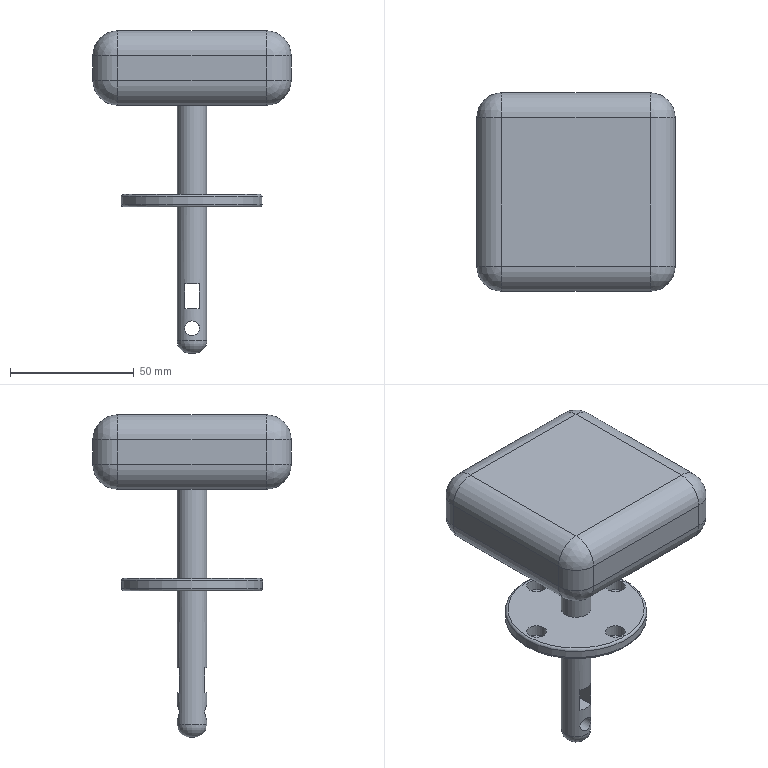Part | STEP file | Anemometer | 1 solid | 52 faces | box 80 x 80 x 130 mm | volume 198324 mm3 | cylinder 24 | plane 17 | sphere 8 | torus 3 | commonest cylinder face diameters 20 x12 4.5 x4 8 x4 12 x2 6 x1 57 x1
STEP:
#1=CARTESIAN_POINT('',(46.,-40.,0.));
#2=VERTEX_POINT('',#1);
#3=CARTESIAN_POINT('',(40.,-40.,0.));
#4=DIRECTION('',(0.,0.,-1.));
#5=DIRECTION('',(1.,0.,0.));
#6=AXIS2_PLACEMENT_3D('',#3,#4,#5);
#7=CIRCLE('',#6,6.);
#8=EDGE_CURVE('',#2,#2,#7,.T.);
#9=ORIENTED_EDGE('',*,*,#8,.T.);
#10=EDGE_LOOP('',(#9));
#11=FACE_OUTER_BOUND('',#10,.T.);
#12=CARTESIAN_POINT('',(34.,-40.,-36.));
#13=VERTEX_POINT('',#12);
#14=CARTESIAN_POINT('',(40.,-40.,-36.));
#15=DIRECTION('',(0.,0.,-1.));
#16=DIRECTION('',(-1.,0.,0.));
#17=AXIS2_PLACEMENT_3D('',#14,#15,#16);
#18=CIRCLE('',#17,6.);
#19=EDGE_CURVE('',#13,#13,#18,.T.);
#20=ORIENTED_EDGE('',*,*,#19,.F.);
#21=EDGE_LOOP('',(#20));
#22=FACE_OUTER_BOUND('',#21,.T.);
#23=CARTESIAN_POINT('',(40.,-40.,-100.));
#24=DIRECTION('',(0.,0.,1.));
#25=DIRECTION('',(1.,0.,0.));
#26=AXIS2_PLACEMENT_3D('',#23,#24,#25);
#27=CYLINDRICAL_SURFACE('',#26,6.);
#28=ADVANCED_FACE('',(#11,#22),#27,.T.);
#29=CARTESIAN_POINT('',(0.,-10.,10.));
#30=VERTEX_POINT('',#29);
#31=CARTESIAN_POINT('',(0.,-70.,10.));
#32=VERTEX_POINT('',#31);
#33=CARTESIAN_POINT('',(0.,0.,10.));
#34=DIRECTION('',(0.,-1.,0.));
#35=VECTOR('',#34,1000.);
#36=LINE('',#33,#35);
#37=EDGE_CURVE('',#30,#32,#36,.T.);
#38=ORIENTED_EDGE('',*,*,#37,.T.);
#39=CARTESIAN_POINT('',(0.,-70.,20.));
#40=VERTEX_POINT('',#39);
#41=CARTESIAN_POINT('',(0.,-70.,30.));
#42=DIRECTION('',(0.,0.,1.));
#43=VECTOR('',#42,1000.);
#44=LINE('',#41,#43);
#45=EDGE_CURVE('',#32,#40,#44,.T.);
#46=ORIENTED_EDGE('',*,*,#45,.T.);
#47=CARTESIAN_POINT('',(0.,-10.,20.));
#48=VERTEX_POINT('',#47);
#49=CARTESIAN_POINT('',(0.,0.,20.));
#50=DIRECTION('',(0.,1.,0.));
#51=VECTOR('',#50,1000.);
#52=LINE('',#49,#51);
#53=EDGE_CURVE('',#40,#48,#52,.T.);
#54=ORIENTED_EDGE('',*,*,#53,.T.);
#55=CARTESIAN_POINT('',(0.,-10.,30.));
#56=DIRECTION('',(0.,0.,-1.));
#57=VECTOR('',#56,1000.);
#58=LINE('',#55,#57);
#59=EDGE_CURVE('',#48,#30,#58,.T.);
#60=ORIENTED_EDGE('',*,*,#59,.T.);
#61=EDGE_LOOP('',(#38,#46,#54,#60));
#62=FACE_OUTER_BOUND('',#61,.T.);
#63=CARTESIAN_POINT('',(0.,0.,30.));
#64=DIRECTION('',(1.,0.,0.));
#65=DIRECTION('',(0.,0.,-1.));
#66=AXIS2_PLACEMENT_3D('',#63,#64,#65);
#67=PLANE('',#66);
#68=ADVANCED_FACE('',(#62),#67,.F.);
#69=CARTESIAN_POINT('',(10.,-80.,20.));
#70=VERTEX_POINT('',#69);
#71=CARTESIAN_POINT('',(10.,-80.,10.));
#72=VERTEX_POINT('',#71);
#73=CARTESIAN_POINT('',(10.,-80.,30.));
#74=DIRECTION('',(0.,0.,-1.));
#75=VECTOR('',#74,1000.);
#76=LINE('',#73,#75);
#77=EDGE_CURVE('',#70,#72,#76,.T.);
#78=ORIENTED_EDGE('',*,*,#77,.T.);
#79=CARTESIAN_POINT('',(70.,-80.,10.));
#80=VERTEX_POINT('',#79);
#81=CARTESIAN_POINT('',(0.,-80.,10.));
#82=DIRECTION('',(1.,0.,0.));
#83=VECTOR('',#82,1000.);
#84=LINE('',#81,#83);
#85=EDGE_CURVE('',#72,#80,#84,.T.);
#86=ORIENTED_EDGE('',*,*,#85,.T.);
#87=CARTESIAN_POINT('',(70.,-80.,20.));
#88=VERTEX_POINT('',#87);
#89=CARTESIAN_POINT('',(70.,-80.,30.));
#90=DIRECTION('',(0.,0.,1.));
#91=VECTOR('',#90,1000.);
#92=LINE('',#89,#91);
#93=EDGE_CURVE('',#80,#88,#92,.T.);
#94=ORIENTED_EDGE('',*,*,#93,.T.);
#95=CARTESIAN_POINT('',(0.,-80.,20.));
#96=DIRECTION('',(-1.,0.,0.));
#97=VECTOR('',#96,1000.);
#98=LINE('',#95,#97);
#99=EDGE_CURVE('',#88,#70,#98,.T.);
#100=ORIENTED_EDGE('',*,*,#99,.T.);
#101=EDGE_LOOP('',(#78,#86,#94,#100));
#102=FACE_OUTER_BOUND('',#101,.T.);
#103=CARTESIAN_POINT('',(0.,-80.,30.));
#104=DIRECTION('',(0.,1.,0.));
#105=DIRECTION('',(0.,0.,1.));
#106=AXIS2_PLACEMENT_3D('',#103,#104,#105);
#107=PLANE('',#106);
#108=ADVANCED_FACE('',(#102),#107,.F.);
#109=CARTESIAN_POINT('',(80.,-10.,20.));
#110=VERTEX_POINT('',#109);
#111=CARTESIAN_POINT('',(80.,-70.,20.));
#112=VERTEX_POINT('',#111);
#113=CARTESIAN_POINT('',(80.,-80.,20.));
#114=DIRECTION('',(0.,-1.,0.));
#115=VECTOR('',#114,1000.);
#116=LINE('',#113,#115);
#117=EDGE_CURVE('',#110,#112,#116,.T.);
#118=ORIENTED_EDGE('',*,*,#117,.T.);
#119=CARTESIAN_POINT('',(80.,-70.,10.));
#120=VERTEX_POINT('',#119);
#121=CARTESIAN_POINT('',(80.,-70.,30.));
#122=DIRECTION('',(0.,0.,-1.));
#123=VECTOR('',#122,1000.);
#124=LINE('',#121,#123);
#125=EDGE_CURVE('',#112,#120,#124,.T.);
#126=ORIENTED_EDGE('',*,*,#125,.T.);
#127=CARTESIAN_POINT('',(80.,-10.,10.));
#128=VERTEX_POINT('',#127);
#129=CARTESIAN_POINT('',(80.,0.,10.));
#130=DIRECTION('',(0.,1.,0.));
#131=VECTOR('',#130,1000.);
#132=LINE('',#129,#131);
#133=EDGE_CURVE('',#120,#128,#132,.T.);
#134=ORIENTED_EDGE('',*,*,#133,.T.);
#135=CARTESIAN_POINT('',(80.,-10.,30.));
#136=DIRECTION('',(0.,0.,1.));
#137=VECTOR('',#136,1000.);
#138=LINE('',#135,#137);
#139=EDGE_CURVE('',#128,#110,#138,.T.);
#140=ORIENTED_EDGE('',*,*,#139,.T.);
#141=EDGE_LOOP('',(#118,#126,#134,#140));
#142=FACE_OUTER_BOUND('',#141,.T.);
#143=CARTESIAN_POINT('',(80.,0.,30.));
#144=DIRECTION('',(-1.,0.,0.));
#145=DIRECTION('',(0.,-1.,0.));
#146=AXIS2_PLACEMENT_3D('',#143,#144,#145);
#147=PLANE('',#146);
#148=ADVANCED_FACE('',(#142),#147,.F.);
#149=CARTESIAN_POINT('',(70.,0.,20.));
#150=VERTEX_POINT('',#149);
#151=CARTESIAN_POINT('',(70.,0.,10.));
#152=VERTEX_POINT('',#151);
#153=CARTESIAN_POINT('',(70.,0.,30.));
#154=DIRECTION('',(0.,0.,-1.));
#155=VECTOR('',#154,1000.);
#156=LINE('',#153,#155);
#157=EDGE_CURVE('',#150,#152,#156,.T.);
#158=ORIENTED_EDGE('',*,*,#157,.T.);
#159=CARTESIAN_POINT('',(10.,0.,10.));
#160=VERTEX_POINT('',#159);
#161=CARTESIAN_POINT('',(0.,0.,10.));
#162=DIRECTION('',(-1.,0.,0.));
#163=VECTOR('',#162,1000.);
#164=LINE('',#161,#163);
#165=EDGE_CURVE('',#152,#160,#164,.T.);
#166=ORIENTED_EDGE('',*,*,#165,.T.);
#167=CARTESIAN_POINT('',(10.,0.,20.));
#168=VERTEX_POINT('',#167);
#169=CARTESIAN_POINT('',(10.,0.,30.));
#170=DIRECTION('',(0.,0.,1.));
#171=VECTOR('',#170,1000.);
#172=LINE('',#169,#171);
#173=EDGE_CURVE('',#160,#168,#172,.T.);
#174=ORIENTED_EDGE('',*,*,#173,.T.);
#175=CARTESIAN_POINT('',(80.,0.,20.));
#176=DIRECTION('',(1.,0.,0.));
#177=VECTOR('',#176,1000.);
#178=LINE('',#175,#177);
#179=EDGE_CURVE('',#168,#150,#178,.T.);
#180=ORIENTED_EDGE('',*,*,#179,.T.);
#181=EDGE_LOOP('',(#158,#166,#174,#180));
#182=FACE_OUTER_BOUND('',#181,.T.);
#183=CARTESIAN_POINT('',(0.,0.,30.));
#184=DIRECTION('',(0.,-1.,0.));
#185=DIRECTION('',(0.,0.,-1.));
#186=AXIS2_PLACEMENT_3D('',#183,#184,#185);
#187=PLANE('',#186);
#188=ADVANCED_FACE('',(#182),#187,.F.);
#189=CARTESIAN_POINT('',(70.,-70.,30.));
#190=VERTEX_POINT('',#189);
#191=CARTESIAN_POINT('',(70.,-10.,30.));
#192=VERTEX_POINT('',#191);
#193=CARTESIAN_POINT('',(70.,0.,30.));
#194=DIRECTION('',(0.,1.,0.));
#195=VECTOR('',#194,1000.);
#196=LINE('',#193,#195);
#197=EDGE_CURVE('',#190,#192,#196,.T.);
#198=ORIENTED_EDGE('',*,*,#197,.T.);
#199=CARTESIAN_POINT('',(10.,-10.,30.));
#200=VERTEX_POINT('',#199);
#201=CARTESIAN_POINT('',(0.,-10.,30.));
#202=DIRECTION('',(-1.,0.,0.));
#203=VECTOR('',#202,1000.);
#204=LINE('',#201,#203);
#205=EDGE_CURVE('',#192,#200,#204,.T.);
#206=ORIENTED_EDGE('',*,*,#205,.T.);
#207=CARTESIAN_POINT('',(10.,-70.,30.));
#208=VERTEX_POINT('',#207);
#209=CARTESIAN_POINT('',(10.,-80.,30.));
#210=DIRECTION('',(0.,-1.,0.));
#211=VECTOR('',#210,1000.);
#212=LINE('',#209,#211);
#213=EDGE_CURVE('',#200,#208,#212,.T.);
#214=ORIENTED_EDGE('',*,*,#213,.T.);
#215=CARTESIAN_POINT('',(80.,-70.,30.));
#216=DIRECTION('',(1.,0.,0.));
#217=VECTOR('',#216,1000.);
#218=LINE('',#215,#217);
#219=EDGE_CURVE('',#208,#190,#218,.T.);
#220=ORIENTED_EDGE('',*,*,#219,.T.);
#221=EDGE_LOOP('',(#198,#206,#214,#220));
#222=FACE_OUTER_BOUND('',#221,.T.);
#223=CARTESIAN_POINT('',(0.,0.,30.));
#224=DIRECTION('',(0.,0.,1.));
#225=DIRECTION('',(1.,0.,0.));
#226=AXIS2_PLACEMENT_3D('',#223,#224,#225);
#227=PLANE('',#226);
#228=ADVANCED_FACE('',(#222),#227,.T.);
#229=ORIENTED_EDGE('',*,*,#8,.F.);
#230=EDGE_LOOP('',(#229));
#231=FACE_BOUND('',#230,.T.);
#232=CARTESIAN_POINT('',(70.,-10.,0.));
#233=VERTEX_POINT('',#232);
#234=CARTESIAN_POINT('',(70.,-70.,0.));
#235=VERTEX_POINT('',#234);
#236=CARTESIAN_POINT('',(70.,0.,0.));
#237=DIRECTION('',(0.,-1.,0.));
#238=VECTOR('',#237,1000.);
#239=LINE('',#236,#238);
#240=EDGE_CURVE('',#233,#235,#239,.T.);
#241=ORIENTED_EDGE('',*,*,#240,.T.);
#242=CARTESIAN_POINT('',(10.,-70.,0.));
#243=VERTEX_POINT('',#242);
#244=CARTESIAN_POINT('',(0.,-70.,0.));
#245=DIRECTION('',(-1.,0.,0.));
#246=VECTOR('',#245,1000.);
#247=LINE('',#244,#246);
#248=EDGE_CURVE('',#235,#243,#247,.T.);
#249=ORIENTED_EDGE('',*,*,#248,.T.);
#250=CARTESIAN_POINT('',(10.,-10.,0.));
#251=VERTEX_POINT('',#250);
#252=CARTESIAN_POINT('',(10.,0.,0.));
#253=DIRECTION('',(0.,1.,0.));
#254=VECTOR('',#253,1000.);
#255=LINE('',#252,#254);
#256=EDGE_CURVE('',#243,#251,#255,.T.);
#257=ORIENTED_EDGE('',*,*,#256,.T.);
#258=CARTESIAN_POINT('',(0.,-10.,0.));
#259=DIRECTION('',(1.,0.,0.));
#260=VECTOR('',#259,1000.);
#261=LINE('',#258,#260);
#262=EDGE_CURVE('',#251,#233,#261,.T.);
#263=ORIENTED_EDGE('',*,*,#262,.T.);
#264=EDGE_LOOP('',(#241,#249,#257,#263));
#265=FACE_OUTER_BOUND('',#264,.T.);
#266=CARTESIAN_POINT('',(0.,0.,0.));
#267=DIRECTION('',(0.,0.,1.));
#268=DIRECTION('',(1.,0.,0.));
#269=AXIS2_PLACEMENT_3D('',#266,#267,#268);
#270=PLANE('',#269);
#271=ADVANCED_FACE('',(#231,#265),#270,.F.);
#272=CARTESIAN_POINT('',(70.,-10.,20.));
#273=DIRECTION('',(0.,0.,1.));
#274=DIRECTION('',(1.,0.,0.));
#275=AXIS2_PLACEMENT_3D('',#272,#273,#274);
#276=CIRCLE('',#275,10.);
#277=EDGE_CURVE('',#110,#150,#276,.T.);
#278=ORIENTED_EDGE('',*,*,#277,.F.);
#279=ORIENTED_EDGE('',*,*,#139,.F.);
#280=CARTESIAN_POINT('',(70.,-10.,10.));
#281=DIRECTION('',(0.,0.,-1.));
#282=DIRECTION('',(-1.,0.,0.));
#283=AXIS2_PLACEMENT_3D('',#280,#281,#282);
#284=CIRCLE('',#283,10.);
#285=EDGE_CURVE('',#152,#128,#284,.T.);
#286=ORIENTED_EDGE('',*,*,#285,.F.);
#287=ORIENTED_EDGE('',*,*,#157,.F.);
#288=EDGE_LOOP('',(#278,#279,#286,#287));
#289=FACE_OUTER_BOUND('',#288,.T.);
#290=CARTESIAN_POINT('',(70.,-10.,30.));
#291=DIRECTION('',(0.,0.,-1.));
#292=DIRECTION('',(-1.,0.,0.));
#293=AXIS2_PLACEMENT_3D('',#290,#291,#292);
#294=CYLINDRICAL_SURFACE('',#293,10.);
#295=ADVANCED_FACE('',(#289),#294,.T.);
#296=CARTESIAN_POINT('',(70.,-10.,20.));
#297=DIRECTION('',(0.,-1.,0.));
#298=DIRECTION('',(-1.,0.,0.));
#299=AXIS2_PLACEMENT_3D('',#296,#297,#298);
#300=CIRCLE('',#299,10.);
#301=EDGE_CURVE('',#110,#192,#300,.T.);
#302=ORIENTED_EDGE('',*,*,#301,.F.);
#303=ORIENTED_EDGE('',*,*,#277,.T.);
#304=CARTESIAN_POINT('',(70.,-10.,20.));
#305=DIRECTION('',(-1.,0.,0.));
#306=DIRECTION('',(0.,0.,-1.));
#307=AXIS2_PLACEMENT_3D('',#304,#305,#306);
#308=CIRCLE('',#307,10.);
#309=EDGE_CURVE('',#192,#150,#308,.T.);
#310=ORIENTED_EDGE('',*,*,#309,.F.);
#311=EDGE_LOOP('',(#302,#303,#310));
#312=FACE_OUTER_BOUND('',#311,.T.);
#313=CARTESIAN_POINT('',(70.,-10.,20.));
#314=DIRECTION('',(0.,1.,0.));
#315=DIRECTION('',(1.,0.,0.));
#316=AXIS2_PLACEMENT_3D('',#313,#314,#315);
#317=SPHERICAL_SURFACE('',#316,10.);
#318=ADVANCED_FACE('',(#312),#317,.T.);
#319=CARTESIAN_POINT('',(70.,-10.,10.));
#320=DIRECTION('',(-1.,0.,0.));
#321=DIRECTION('',(0.,0.,-1.));
#322=AXIS2_PLACEMENT_3D('',#319,#320,#321);
#323=CIRCLE('',#322,10.);
#324=EDGE_CURVE('',#152,#233,#323,.T.);
#325=ORIENTED_EDGE('',*,*,#324,.F.);
#326=ORIENTED_EDGE('',*,*,#285,.T.);
#327=CARTESIAN_POINT('',(70.,-10.,10.));
#328=DIRECTION('',(0.,-1.,0.));
#329=DIRECTION('',(-1.,0.,0.));
#330=AXIS2_PLACEMENT_3D('',#327,#328,#329);
#331=CIRCLE('',#330,10.);
#332=EDGE_CURVE('',#233,#128,#331,.T.);
#333=ORIENTED_EDGE('',*,*,#332,.F.);
#334=EDGE_LOOP('',(#325,#326,#333));
#335=FACE_OUTER_BOUND('',#334,.T.);
#336=CARTESIAN_POINT('',(70.,-10.,10.));
#337=DIRECTION('',(0.,1.,0.));
#338=DIRECTION('',(1.,0.,0.));
#339=AXIS2_PLACEMENT_3D('',#336,#337,#338);
#340=SPHERICAL_SURFACE('',#339,10.);
#341=ADVANCED_FACE('',(#335),#340,.T.);
#342=ORIENTED_EDGE('',*,*,#309,.T.);
#343=ORIENTED_EDGE('',*,*,#179,.F.);
#344=CARTESIAN_POINT('',(10.,-10.,20.));
#345=DIRECTION('',(-1.,0.,0.));
#346=DIRECTION('',(0.,0.,1.));
#347=AXIS2_PLACEMENT_3D('',#344,#345,#346);
#348=CIRCLE('',#347,10.);
#349=EDGE_CURVE('',#200,#168,#348,.T.);
#350=ORIENTED_EDGE('',*,*,#349,.F.);
#351=ORIENTED_EDGE('',*,*,#205,.F.);
#352=EDGE_LOOP('',(#342,#343,#350,#351));
#353=FACE_OUTER_BOUND('',#352,.T.);
#354=CARTESIAN_POINT('',(0.,-10.,20.));
#355=DIRECTION('',(1.,0.,0.));
#356=DIRECTION('',(0.,0.,-1.));
#357=AXIS2_PLACEMENT_3D('',#354,#355,#356);
#358=CYLINDRICAL_SURFACE('',#357,10.);
#359=ADVANCED_FACE('',(#353),#358,.T.);
#360=ORIENTED_EDGE('',*,*,#301,.T.);
#361=ORIENTED_EDGE('',*,*,#197,.F.);
#362=CARTESIAN_POINT('',(70.,-70.,20.));
#363=DIRECTION('',(0.,-1.,0.));
#364=DIRECTION('',(0.,0.,-1.));
#365=AXIS2_PLACEMENT_3D('',#362,#363,#364);
#366=CIRCLE('',#365,10.);
#367=EDGE_CURVE('',#112,#190,#366,.T.);
#368=ORIENTED_EDGE('',*,*,#367,.F.);
#369=ORIENTED_EDGE('',*,*,#117,.F.);
#370=EDGE_LOOP('',(#360,#361,#368,#369));
#371=FACE_OUTER_BOUND('',#370,.T.);
#372=CARTESIAN_POINT('',(70.,0.,20.));
#373=DIRECTION('',(0.,-1.,0.));
#374=DIRECTION('',(1.,0.,0.));
#375=AXIS2_PLACEMENT_3D('',#372,#373,#374);
#376=CYLINDRICAL_SURFACE('',#375,10.);
#377=ADVANCED_FACE('',(#371),#376,.T.);
#378=CARTESIAN_POINT('',(70.,-70.,10.));
#379=DIRECTION('',(0.,0.,-1.));
#380=DIRECTION('',(-1.,0.,0.));
#381=AXIS2_PLACEMENT_3D('',#378,#379,#380);
#382=CIRCLE('',#381,10.);
#383=EDGE_CURVE('',#120,#80,#382,.T.);
#384=ORIENTED_EDGE('',*,*,#383,.F.);
#385=ORIENTED_EDGE('',*,*,#125,.F.);
#386=CARTESIAN_POINT('',(70.,-70.,20.));
#387=DIRECTION('',(0.,0.,1.));
#388=DIRECTION('',(1.,0.,0.));
#389=AXIS2_PLACEMENT_3D('',#386,#387,#388);
#390=CIRCLE('',#389,10.);
#391=EDGE_CURVE('',#88,#112,#390,.T.);
#392=ORIENTED_EDGE('',*,*,#391,.F.);
#393=ORIENTED_EDGE('',*,*,#93,.F.);
#394=EDGE_LOOP('',(#384,#385,#392,#393));
#395=FACE_OUTER_BOUND('',#394,.T.);
#396=CARTESIAN_POINT('',(70.,-70.,30.));
#397=DIRECTION('',(0.,0.,-1.));
#398=DIRECTION('',(-1.,0.,0.));
#399=AXIS2_PLACEMENT_3D('',#396,#397,#398);
#400=CYLINDRICAL_SURFACE('',#399,10.);
#401=ADVANCED_FACE('',(#395),#400,.T.);
#402=ORIENTED_EDGE('',*,*,#332,.T.);
#403=ORIENTED_EDGE('',*,*,#133,.F.);
#404=CARTESIAN_POINT('',(70.,-70.,10.));
#405=DIRECTION('',(0.,-1.,0.));
#406=DIRECTION('',(0.,0.,-1.));
#407=AXIS2_PLACEMENT_3D('',#404,#405,#406);
#408=CIRCLE('',#407,10.);
#409=EDGE_CURVE('',#235,#120,#408,.T.);
#410=ORIENTED_EDGE('',*,*,#409,.F.);
#411=ORIENTED_EDGE('',*,*,#240,.F.);
#412=EDGE_LOOP('',(#402,#403,#410,#411));
#413=FACE_OUTER_BOUND('',#412,.T.);
#414=CARTESIAN_POINT('',(70.,0.,10.));
#415=DIRECTION('',(0.,1.,0.));
#416=DIRECTION('',(-1.,0.,0.));
#417=AXIS2_PLACEMENT_3D('',#414,#415,#416);
#418=CYLINDRICAL_SURFACE('',#417,10.);
#419=ADVANCED_FACE('',(#413),#418,.T.);
#420=ORIENTED_EDGE('',*,*,#324,.T.);
#421=ORIENTED_EDGE('',*,*,#262,.F.);
#422=CARTESIAN_POINT('',(10.,-10.,10.));
#423=DIRECTION('',(-1.,0.,0.));
#424=DIRECTION('',(0.,0.,1.));
#425=AXIS2_PLACEMENT_3D('',#422,#423,#424);
#426=CIRCLE('',#425,10.);
#427=EDGE_CURVE('',#160,#251,#426,.T.);
#428=ORIENTED_EDGE('',*,*,#427,.F.);
#429=ORIENTED_EDGE('',*,*,#165,.F.);
#430=EDGE_LOOP('',(#420,#421,#428,#429));
#431=FACE_OUTER_BOUND('',#430,.T.);
#432=CARTESIAN_POINT('',(0.,-10.,10.));
#433=DIRECTION('',(-1.,0.,0.));
#434=DIRECTION('',(0.,0.,1.));
#435=AXIS2_PLACEMENT_3D('',#432,#433,#434);
#436=CYLINDRICAL_SURFACE('',#435,10.);
#437=ADVANCED_FACE('',(#431),#436,.T.);
#438=CARTESIAN_POINT('',(10.,-10.,20.));
#439=DIRECTION('',(0.,0.,1.));
#440=DIRECTION('',(1.,0.,0.));
#441=AXIS2_PLACEMENT_3D('',#438,#439,#440);
#442=CIRCLE('',#441,10.);
#443=EDGE_CURVE('',#168,#48,#442,.T.);
#444=ORIENTED_EDGE('',*,*,#443,.F.);
#445=ORIENTED_EDGE('',*,*,#173,.F.);
#446=CARTESIAN_POINT('',(10.,-10.,10.));
#447=DIRECTION('',(0.,0.,-1.));
#448=DIRECTION('',(-1.,0.,0.));
#449=AXIS2_PLACEMENT_3D('',#446,#447,#448);
#450=CIRCLE('',#449,10.);
#451=EDGE_CURVE('',#30,#160,#450,.T.);
#452=ORIENTED_EDGE('',*,*,#451,.F.);
#453=ORIENTED_EDGE('',*,*,#59,.F.);
#454=EDGE_LOOP('',(#444,#445,#452,#453));
#455=FACE_OUTER_BOUND('',#454,.T.);
#456=CARTESIAN_POINT('',(10.,-10.,30.));
#457=DIRECTION('',(0.,0.,-1.));
#458=DIRECTION('',(-1.,0.,0.));
#459=AXIS2_PLACEMENT_3D('',#456,#457,#458);
#460=CYLINDRICAL_SURFACE('',#459,10.);
#461=ADVANCED_FACE('',(#455),#460,.T.);
#462=ORIENTED_EDGE('',*,*,#349,.T.);
#463=ORIENTED_EDGE('',*,*,#443,.T.);
#464=CARTESIAN_POINT('',(10.,-10.,20.));
#465=DIRECTION('',(0.,-1.,0.));
#466=DIRECTION('',(0.,0.,1.));
#467=AXIS2_PLACEMENT_3D('',#464,#465,#466);
#468=CIRCLE('',#467,10.);
#469=EDGE_CURVE('',#200,#48,#468,.T.);
#470=ORIENTED_EDGE('',*,*,#469,.F.);
#471=EDGE_LOOP('',(#462,#463,#470));
#472=FACE_OUTER_BOUND('',#471,.T.);
#473=CARTESIAN_POINT('',(10.,-10.,20.));
#474=DIRECTION('',(0.,1.,0.));
#475=DIRECTION('',(1.,0.,0.));
#476=AXIS2_PLACEMENT_3D('',#473,#474,#475);
#477=SPHERICAL_SURFACE('',#476,10.);
#478=ADVANCED_FACE('',(#472),#477,.T.);
#479=ORIENTED_EDGE('',*,*,#391,.T.);
#480=ORIENTED_EDGE('',*,*,#367,.T.);
#481=CARTESIAN_POINT('',(70.,-70.,20.));
#482=DIRECTION('',(-1.,0.,0.));
#483=DIRECTION('',(0.,0.,-1.));
#484=AXIS2_PLACEMENT_3D('',#481,#482,#483);
#485=CIRCLE('',#484,10.);
#486=EDGE_CURVE('',#88,#190,#485,.T.);
#487=ORIENTED_EDGE('',*,*,#486,.F.);
#488=EDGE_LOOP('',(#479,#480,#487));
#489=FACE_OUTER_BOUND('',#488,.T.);
#490=CARTESIAN_POINT('',(70.,-70.,20.));
#491=DIRECTION('',(0.,1.,0.));
#492=DIRECTION('',(1.,0.,0.));
#493=AXIS2_PLACEMENT_3D('',#490,#491,#492);
#494=SPHERICAL_SURFACE('',#493,10.);
#495=ADVANCED_FACE('',(#489),#494,.T.);
#496=ORIENTED_EDGE('',*,*,#409,.T.);
#497=ORIENTED_EDGE('',*,*,#383,.T.);
#498=CARTESIAN_POINT('',(70.,-70.,10.));
#499=DIRECTION('',(-1.,0.,0.));
#500=DIRECTION('',(0.,0.,-1.));
#501=AXIS2_PLACEMENT_3D('',#498,#499,#500);
#502=CIRCLE('',#501,10.);
#503=EDGE_CURVE('',#235,#80,#502,.T.);
#504=ORIENTED_EDGE('',*,*,#503,.F.);
#505=EDGE_LOOP('',(#496,#497,#504));
#506=FACE_OUTER_BOUND('',#505,.T.);
#507=CARTESIAN_POINT('',(70.,-70.,10.));
#508=DIRECTION('',(0.,1.,0.));
#509=DIRECTION('',(1.,0.,0.));
#510=AXIS2_PLACEMENT_3D('',#507,#508,#509);
#511=SPHERICAL_SURFACE('',#510,10.);
#512=ADVANCED_FACE('',(#506),#511,.T.);
#513=ORIENTED_EDGE('',*,*,#451,.T.);
#514=ORIENTED_EDGE('',*,*,#427,.T.);
#515=CARTESIAN_POINT('',(10.,-10.,10.));
#516=DIRECTION('',(0.,-1.,0.));
#517=DIRECTION('',(0.,0.,1.));
#518=AXIS2_PLACEMENT_3D('',#515,#516,#517);
#519=CIRCLE('',#518,10.);
#520=EDGE_CURVE('',#30,#251,#519,.T.);
#521=ORIENTED_EDGE('',*,*,#520,.F.);
#522=EDGE_LOOP('',(#513,#514,#521));
#523=FACE_OUTER_BOUND('',#522,.T.);
#524=CARTESIAN_POINT('',(10.,-10.,10.));
#525=DIRECTION('',(0.,1.,0.));
#526=DIRECTION('',(1.,0.,0.));
#527=AXIS2_PLACEMENT_3D('',#524,#525,#526);
#528=SPHERICAL_SURFACE('',#527,10.);
#529=ADVANCED_FACE('',(#523),#528,.T.);
#530=ORIENTED_EDGE('',*,*,#469,.T.);
#531=ORIENTED_EDGE('',*,*,#53,.F.);
#532=CARTESIAN_POINT('',(10.,-70.,20.));
#533=DIRECTION('',(0.,-1.,0.));
#534=DIRECTION('',(0.,0.,-1.));
#535=AXIS2_PLACEMENT_3D('',#532,#533,#534);
#536=CIRCLE('',#535,10.);
#537=EDGE_CURVE('',#208,#40,#536,.T.);
#538=ORIENTED_EDGE('',*,*,#537,.F.);
#539=ORIENTED_EDGE('',*,*,#213,.F.);
#540=EDGE_LOOP('',(#530,#531,#538,#539));
#541=FACE_OUTER_BOUND('',#540,.T.);
#542=CARTESIAN_POINT('',(10.,0.,20.));
#543=DIRECTION('',(0.,1.,0.));
#544=DIRECTION('',(0.,0.,1.));
#545=AXIS2_PLACEMENT_3D('',#542,#543,#544);
#546=CYLINDRICAL_SURFACE('',#545,10.);
#547=ADVANCED_FACE('',(#541),#546,.T.);
#548=ORIENTED_EDGE('',*,*,#486,.T.);
#549=ORIENTED_EDGE('',*,*,#219,.F.);
#550=CARTESIAN_POINT('',(10.,-70.,20.));
#551=DIRECTION('',(-1.,0.,0.));
#552=DIRECTION('',(0.,0.,1.));
#553=AXIS2_PLACEMENT_3D('',#550,#551,#552);
#554=CIRCLE('',#553,10.);
#555=EDGE_CURVE('',#70,#208,#554,.T.);
#556=ORIENTED_EDGE('',*,*,#555,.F.);
#557=ORIENTED_EDGE('',*,*,#99,.F.);
#558=EDGE_LOOP('',(#548,#549,#556,#557));
#559=FACE_OUTER_BOUND('',#558,.T.);
#560=CARTESIAN_POINT('',(0.,-70.,20.));
#561=DIRECTION('',(-1.,0.,0.));
#562=DIRECTION('',(0.,0.,1.));
#563=AXIS2_PLACEMENT_3D('',#560,#561,#562);
#564=CYLINDRICAL_SURFACE('',#563,10.);
#565=ADVANCED_FACE('',(#559),#564,.T.);
#566=ORIENTED_EDGE('',*,*,#503,.T.);
#567=ORIENTED_EDGE('',*,*,#85,.F.);
#568=CARTESIAN_POINT('',(10.,-70.,10.));
#569=DIRECTION('',(-1.,0.,0.));
#570=DIRECTION('',(0.,0.,1.));
#571=AXIS2_PLACEMENT_3D('',#568,#569,#570);
#572=CIRCLE('',#571,10.);
#573=EDGE_CURVE('',#243,#72,#572,.T.);
#574=ORIENTED_EDGE('',*,*,#573,.F.);
#575=ORIENTED_EDGE('',*,*,#248,.F.);
#576=EDGE_LOOP('',(#566,#567,#574,#575));
#577=FACE_OUTER_BOUND('',#576,.T.);
#578=CARTESIAN_POINT('',(0.,-70.,10.));
#579=DIRECTION('',(1.,0.,0.));
#580=DIRECTION('',(0.,0.,-1.));
#581=AXIS2_PLACEMENT_3D('',#578,#579,#580);
#582=CYLINDRICAL_SURFACE('',#581,10.);
#583=ADVANCED_FACE('',(#577),#582,.T.);
#584=ORIENTED_EDGE('',*,*,#520,.T.);
#585=ORIENTED_EDGE('',*,*,#256,.F.);
#586=CARTESIAN_POINT('',(10.,-70.,10.));
#587=DIRECTION('',(0.,-1.,0.));
#588=DIRECTION('',(0.,0.,-1.));
#589=AXIS2_PLACEMENT_3D('',#586,#587,#588);
#590=CIRCLE('',#589,10.);
#591=EDGE_CURVE('',#32,#243,#590,.T.);
#592=ORIENTED_EDGE('',*,*,#591,.F.);
#593=ORIENTED_EDGE('',*,*,#37,.F.);
#594=EDGE_LOOP('',(#584,#585,#592,#593));
#595=FACE_OUTER_BOUND('',#594,.T.);
#596=CARTESIAN_POINT('',(10.,0.,10.));
#597=DIRECTION('',(0.,-1.,0.));
#598=DIRECTION('',(0.,0.,-1.));
#599=AXIS2_PLACEMENT_3D('',#596,#597,#598);
#600=CYLINDRICAL_SURFACE('',#599,10.);
#601=ADVANCED_FACE('',(#595),#600,.T.);
#602=ORIENTED_EDGE('',*,*,#555,.T.);
#603=ORIENTED_EDGE('',*,*,#537,.T.);
#604=CARTESIAN_POINT('',(10.,-70.,20.));
#605=DIRECTION('',(0.,0.,-1.));
#606=DIRECTION('',(1.,0.,0.));
#607=AXIS2_PLACEMENT_3D('',#604,#605,#606);
#608=CIRCLE('',#607,10.);
#609=EDGE_CURVE('',#70,#40,#608,.T.);
#610=ORIENTED_EDGE('',*,*,#609,.F.);
#611=EDGE_LOOP('',(#602,#603,#610));
#612=FACE_OUTER_BOUND('',#611,.T.);
#613=CARTESIAN_POINT('',(10.,-70.,20.));
#614=DIRECTION('',(0.,1.,0.));
#615=DIRECTION('',(1.,0.,0.));
#616=AXIS2_PLACEMENT_3D('',#613,#614,#615);
#617=SPHERICAL_SURFACE('',#616,10.);
#618=ADVANCED_FACE('',(#612),#617,.T.);
#619=ORIENTED_EDGE('',*,*,#591,.T.);
#620=ORIENTED_EDGE('',*,*,#573,.T.);
#621=CARTESIAN_POINT('',(10.,-70.,10.));
#622=DIRECTION('',(0.,0.,1.));
#623=DIRECTION('',(-1.,0.,0.));
#624=AXIS2_PLACEMENT_3D('',#621,#622,#623);
#625=CIRCLE('',#624,10.);
#626=EDGE_CURVE('',#32,#72,#625,.T.);
#627=ORIENTED_EDGE('',*,*,#626,.F.);
#628=EDGE_LOOP('',(#619,#620,#627));
#629=FACE_OUTER_BOUND('',#628,.T.);
#630=CARTESIAN_POINT('',(10.,-70.,10.));
#631=DIRECTION('',(0.,1.,0.));
#632=DIRECTION('',(1.,0.,0.));
#633=AXIS2_PLACEMENT_3D('',#630,#631,#632);
#634=SPHERICAL_SURFACE('',#633,10.);
#635=ADVANCED_FACE('',(#629),#634,.T.);
#636=ORIENTED_EDGE('',*,*,#609,.T.);
#637=ORIENTED_EDGE('',*,*,#45,.F.);
#638=ORIENTED_EDGE('',*,*,#626,.T.);
#639=ORIENTED_EDGE('',*,*,#77,.F.);
#640=EDGE_LOOP('',(#636,#637,#638,#639));
#641=FACE_OUTER_BOUND('',#640,.T.);
#642=CARTESIAN_POINT('',(10.,-70.,30.));
#643=DIRECTION('',(0.,0.,-1.));
#644=DIRECTION('',(-1.,0.,0.));
#645=AXIS2_PLACEMENT_3D('',#642,#643,#644);
#646=CYLINDRICAL_SURFACE('',#645,10.);
#647=ADVANCED_FACE('',(#641),#646,.T.);
#648=CARTESIAN_POINT('',(11.5,-40.,-37.));
#649=VERTEX_POINT('',#648);
#650=CARTESIAN_POINT('',(40.,-40.,-37.));
#651=DIRECTION('',(0.,0.,-1.));
#652=DIRECTION('',(-1.,0.,0.));
#653=AXIS2_PLACEMENT_3D('',#650,#651,#652);
#654=CIRCLE('',#653,28.5);
#655=EDGE_CURVE('',#649,#649,#654,.T.);
#656=ORIENTED_EDGE('',*,*,#655,.T.);
#657=EDGE_LOOP('',(#656));
#658=FACE_OUTER_BOUND('',#657,.T.);
#659=CARTESIAN_POINT('',(11.5,-40.,-40.));
#660=VERTEX_POINT('',#659);
#661=CARTESIAN_POINT('',(40.,-40.,-40.));
#662=DIRECTION('',(0.,0.,1.));
#663=DIRECTION('',(-1.,0.,0.));
#664=AXIS2_PLACEMENT_3D('',#661,#662,#663);
#665=CIRCLE('',#664,28.5);
#666=EDGE_CURVE('',#660,#660,#665,.T.);
#667=ORIENTED_EDGE('',*,*,#666,.T.);
#668=EDGE_LOOP('',(#667));
#669=FACE_OUTER_BOUND('',#668,.T.);
#670=CARTESIAN_POINT('',(40.,-40.,-41.));
#671=DIRECTION('',(0.,0.,1.));
#672=DIRECTION('',(1.,0.,0.));
#673=AXIS2_PLACEMENT_3D('',#670,#671,#672);
#674=CYLINDRICAL_SURFACE('',#673,28.5);
#675=ADVANCED_FACE('',(#658,#669),#674,.T.);
#676=CARTESIAN_POINT('',(37.75,-17.5,-41.));
#677=VERTEX_POINT('',#676);
#678=CARTESIAN_POINT('',(40.,-17.5,-41.));
#679=DIRECTION('',(0.,0.,-1.));
#680=DIRECTION('',(-1.,0.,0.));
#681=AXIS2_PLACEMENT_3D('',#678,#679,#680);
#682=CIRCLE('',#681,2.25);
#683=EDGE_CURVE('',#677,#677,#682,.T.);
#684=ORIENTED_EDGE('',*,*,#683,.F.);
#685=EDGE_LOOP('',(#684));
#686=FACE_BOUND('',#685,.T.);
#687=CARTESIAN_POINT('',(60.25,-40.,-41.));
#688=VERTEX_POINT('',#687);
#689=CARTESIAN_POINT('',(62.5,-40.,-41.));
#690=DIRECTION('',(0.,0.,-1.));
#691=DIRECTION('',(-1.,0.,0.));
#692=AXIS2_PLACEMENT_3D('',#689,#690,#691);
#693=CIRCLE('',#692,2.25);
#694=EDGE_CURVE('',#688,#688,#693,.T.);
#695=ORIENTED_EDGE('',*,*,#694,.F.);
#696=EDGE_LOOP('',(#695));
#697=FACE_BOUND('',#696,.T.);
#698=CARTESIAN_POINT('',(37.75,-62.5,-41.));
#699=VERTEX_POINT('',#698);
#700=CARTESIAN_POINT('',(40.,-62.5,-41.));
#701=DIRECTION('',(0.,0.,-1.));
#702=DIRECTION('',(-1.,0.,0.));
#703=AXIS2_PLACEMENT_3D('',#700,#701,#702);
#704=CIRCLE('',#703,2.25);
#705=EDGE_CURVE('',#699,#699,#704,.T.);
#706=ORIENTED_EDGE('',*,*,#705,.F.);
#707=EDGE_LOOP('',(#706));
#708=FACE_BOUND('',#707,.T.);
#709=CARTESIAN_POINT('',(15.25,-40.,-41.));
#710=VERTEX_POINT('',#709);
#711=CARTESIAN_POINT('',(17.5,-40.,-41.));
#712=DIRECTION('',(0.,0.,-1.));
#713=DIRECTION('',(-1.,0.,0.));
#714=AXIS2_PLACEMENT_3D('',#711,#712,#713);
#715=CIRCLE('',#714,2.25);
#716=EDGE_CURVE('',#710,#710,#715,.T.);
#717=ORIENTED_EDGE('',*,*,#716,.F.);
#718=EDGE_LOOP('',(#717));
#719=FACE_BOUND('',#718,.T.);
#720=CARTESIAN_POINT('',(12.5,-40.,-41.));
#721=VERTEX_POINT('',#720);
#722=CARTESIAN_POINT('',(40.,-40.,-41.));
#723=DIRECTION('',(0.,0.,-1.));
#724=DIRECTION('',(-1.,0.,0.));
#725=AXIS2_PLACEMENT_3D('',#722,#723,#724);
#726=CIRCLE('',#725,27.5);
#727=EDGE_CURVE('',#721,#721,#726,.T.);
#728=ORIENTED_EDGE('',*,*,#727,.T.);
#729=EDGE_LOOP('',(#728));
#730=FACE_OUTER_BOUND('',#729,.T.);
#731=CARTESIAN_POINT('',(34.,-40.,-41.));
#732=VERTEX_POINT('',#731);
#733=CARTESIAN_POINT('',(40.,-40.,-41.));
#734=DIRECTION('',(0.,0.,-1.));
#735=DIRECTION('',(-1.,0.,0.));
#736=AXIS2_PLACEMENT_3D('',#733,#734,#735);
#737=CIRCLE('',#736,6.);
#738=EDGE_CURVE('',#732,#732,#737,.T.);
#739=ORIENTED_EDGE('',*,*,#738,.F.);
#740=EDGE_LOOP('',(#739));
#741=FACE_BOUND('',#740,.T.);
#742=CARTESIAN_POINT('',(40.,-40.,-41.));
#743=DIRECTION('',(0.,0.,-1.));
#744=DIRECTION('',(-1.,0.,0.));
#745=AXIS2_PLACEMENT_3D('',#742,#743,#744);
#746=PLANE('',#745);
#747=ADVANCED_FACE('',(#686,#697,#708,#719,#730,#741),#746,.T.);
#748=CARTESIAN_POINT('',(44.,-17.5,-36.));
#749=VERTEX_POINT('',#748);
#750=CARTESIAN_POINT('',(40.,-17.5,-36.));
#751=DIRECTION('',(0.,0.,1.));
#752=DIRECTION('',(1.,0.,0.));
#753=AXIS2_PLACEMENT_3D('',#750,#751,#752);
#754=CIRCLE('',#753,4.);
#755=EDGE_CURVE('',#749,#749,#754,.T.);
#756=ORIENTED_EDGE('',*,*,#755,.F.);
#757=EDGE_LOOP('',(#756));
#758=FACE_BOUND('',#757,.T.);
#759=CARTESIAN_POINT('',(66.5,-40.,-36.));
#760=VERTEX_POINT('',#759);
#761=CARTESIAN_POINT('',(62.5,-40.,-36.));
#762=DIRECTION('',(0.,0.,1.));
#763=DIRECTION('',(1.,0.,0.));
#764=AXIS2_PLACEMENT_3D('',#761,#762,#763);
#765=CIRCLE('',#764,4.);
#766=EDGE_CURVE('',#760,#760,#765,.T.);
#767=ORIENTED_EDGE('',*,*,#766,.F.);
#768=EDGE_LOOP('',(#767));
#769=FACE_BOUND('',#768,.T.);
#770=CARTESIAN_POINT('',(44.,-62.5,-36.));
#771=VERTEX_POINT('',#770);
#772=CARTESIAN_POINT('',(40.,-62.5,-36.));
#773=DIRECTION('',(0.,0.,1.));
#774=DIRECTION('',(1.,0.,0.));
#775=AXIS2_PLACEMENT_3D('',#772,#773,#774);
#776=CIRCLE('',#775,4.);
#777=EDGE_CURVE('',#771,#771,#776,.T.);
#778=ORIENTED_EDGE('',*,*,#777,.F.);
#779=EDGE_LOOP('',(#778));
#780=FACE_BOUND('',#779,.T.);
#781=CARTESIAN_POINT('',(21.5,-40.,-36.));
#782=VERTEX_POINT('',#781);
#783=CARTESIAN_POINT('',(17.5,-40.,-36.));
#784=DIRECTION('',(0.,0.,1.));
#785=DIRECTION('',(1.,0.,0.));
#786=AXIS2_PLACEMENT_3D('',#783,#784,#785);
#787=CIRCLE('',#786,4.);
#788=EDGE_CURVE('',#782,#782,#787,.T.);
#789=ORIENTED_EDGE('',*,*,#788,.F.);
#790=EDGE_LOOP('',(#789));
#791=FACE_BOUND('',#790,.T.);
#792=CARTESIAN_POINT('',(12.5,-40.,-36.));
#793=VERTEX_POINT('',#792);
#794=CARTESIAN_POINT('',(40.,-40.,-36.));
#795=DIRECTION('',(0.,0.,1.));
#796=DIRECTION('',(-1.,0.,0.));
#797=AXIS2_PLACEMENT_3D('',#794,#795,#796);
#798=CIRCLE('',#797,27.5);
#799=EDGE_CURVE('',#793,#793,#798,.T.);
#800=ORIENTED_EDGE('',*,*,#799,.T.);
#801=EDGE_LOOP('',(#800));
#802=FACE_OUTER_BOUND('',#801,.T.);
#803=ORIENTED_EDGE('',*,*,#19,.T.);
#804=EDGE_LOOP('',(#803));
#805=FACE_BOUND('',#804,.T.);
#806=CARTESIAN_POINT('',(40.,-40.,-36.));
#807=DIRECTION('',(0.,0.,-1.));
#808=DIRECTION('',(-1.,0.,0.));
#809=AXIS2_PLACEMENT_3D('',#806,#807,#808);
#810=PLANE('',#809);
#811=ADVANCED_FACE('',(#758,#769,#780,#791,#802,#805),#810,.F.);
#812=CARTESIAN_POINT('',(39.,-40.,-100.));
#813=VERTEX_POINT('',#812);
#814=CARTESIAN_POINT('',(40.,-40.,-100.));
#815=DIRECTION('',(0.,0.,-1.));
#816=DIRECTION('',(-1.,0.,0.));
#817=AXIS2_PLACEMENT_3D('',#814,#815,#816);
#818=CIRCLE('',#817,1.);
#819=EDGE_CURVE('',#813,#813,#818,.T.);
#820=ORIENTED_EDGE('',*,*,#819,.T.);
#821=EDGE_LOOP('',(#820));
#822=FACE_OUTER_BOUND('',#821,.T.);
#823=CARTESIAN_POINT('',(40.,-40.,-100.));
#824=DIRECTION('',(0.,0.,-1.));
#825=DIRECTION('',(-1.,0.,0.));
#826=AXIS2_PLACEMENT_3D('',#823,#824,#825);
#827=PLANE('',#826);
#828=ADVANCED_FACE('',(#822),#827,.T.);
#829=CARTESIAN_POINT('',(34.,-40.,-95.));
#830=VERTEX_POINT('',#829);
#831=CARTESIAN_POINT('',(40.,-40.,-95.));
#832=DIRECTION('',(0.,0.,1.));
#833=DIRECTION('',(-1.,0.,0.));
#834=AXIS2_PLACEMENT_3D('',#831,#832,#833);
#835=CIRCLE('',#834,6.);
#836=EDGE_CURVE('',#830,#830,#835,.T.);
#837=ORIENTED_EDGE('',*,*,#836,.F.);
#838=EDGE_LOOP('',(#837));
#839=FACE_OUTER_BOUND('',#838,.T.);
#840=ORIENTED_EDGE('',*,*,#819,.F.);
#841=EDGE_LOOP('',(#840));
#842=FACE_OUTER_BOUND('',#841,.T.);
#843=CARTESIAN_POINT('',(40.,-40.,-95.));
#844=DIRECTION('',(0.,0.,-1.));
#845=DIRECTION('',(-1.,0.,0.));
#846=AXIS2_PLACEMENT_3D('',#843,#844,#845);
#847=TOROIDAL_SURFACE('',#846,1.,5.);
#848=ADVANCED_FACE('',(#839,#842),#847,.T.);
#849=CARTESIAN_POINT('',(43.,-45.196,-82.));
#850=VERTEX_POINT('',#849);
#851=CARTESIAN_POINT('',(43.,-34.804,-82.));
#852=VERTEX_POINT('',#851);
#853=CARTESIAN_POINT('',(43.,-80.,-82.));
#854=DIRECTION('',(0.,1.,0.));
#855=VECTOR('',#854,1000.);
#856=LINE('',#853,#855);
#857=EDGE_CURVE('',#850,#852,#856,.T.);
#858=ORIENTED_EDGE('',*,*,#857,.F.);
#859=CARTESIAN_POINT('',(43.,-45.196,-72.));
#860=VERTEX_POINT('',#859);
#861=CARTESIAN_POINT('',(43.,-45.196,-100.));
#862=DIRECTION('',(0.,0.,-1.));
#863=VECTOR('',#862,1000.);
#864=LINE('',#861,#863);
#865=EDGE_CURVE('',#860,#850,#864,.T.);
#866=ORIENTED_EDGE('',*,*,#865,.F.);
#867=CARTESIAN_POINT('',(43.,-34.804,-72.));
#868=VERTEX_POINT('',#867);
#869=CARTESIAN_POINT('',(43.,-80.,-72.));
#870=DIRECTION('',(0.,1.,0.));
#871=VECTOR('',#870,1000.);
#872=LINE('',#869,#871);
#873=EDGE_CURVE('',#860,#868,#872,.T.);
#874=ORIENTED_EDGE('',*,*,#873,.T.);
#875=CARTESIAN_POINT('',(43.,-34.804,-100.));
#876=DIRECTION('',(0.,0.,1.));
#877=VECTOR('',#876,1000.);
#878=LINE('',#875,#877);
#879=EDGE_CURVE('',#852,#868,#878,.T.);
#880=ORIENTED_EDGE('',*,*,#879,.F.);
#881=EDGE_LOOP('',(#858,#866,#874,#880));
#882=FACE_OUTER_BOUND('',#881,.T.);
#883=CARTESIAN_POINT('',(43.,-80.,-82.));
#884=DIRECTION('',(1.,0.,0.));
#885=DIRECTION('',(0.,0.,-1.));
#886=AXIS2_PLACEMENT_3D('',#883,#884,#885);
#887=PLANE('',#886);
#888=ADVANCED_FACE('',(#882),#887,.F.);
#889=CARTESIAN_POINT('',(37.,-45.196,-82.));
#890=VERTEX_POINT('',#889);
#891=CARTESIAN_POINT('',(37.,-34.804,-82.));
#892=VERTEX_POINT('',#891);
#893=CARTESIAN_POINT('',(37.,-80.,-82.));
#894=DIRECTION('',(0.,1.,0.));
#895=VECTOR('',#894,1000.);
#896=LINE('',#893,#895);
#897=EDGE_CURVE('',#890,#892,#896,.T.);
#898=ORIENTED_EDGE('',*,*,#897,.F.);
#899=CARTESIAN_POINT('',(40.,-40.,-82.));
#900=DIRECTION('',(0.,0.,-1.));
#901=DIRECTION('',(-1.,0.,0.));
#902=AXIS2_PLACEMENT_3D('',#899,#900,#901);
#903=CIRCLE('',#902,6.);
#904=EDGE_CURVE('',#850,#890,#903,.T.);
#905=ORIENTED_EDGE('',*,*,#904,.F.);
#906=ORIENTED_EDGE('',*,*,#857,.T.);
#907=CARTESIAN_POINT('',(40.,-40.,-82.));
#908=DIRECTION('',(0.,0.,-1.));
#909=DIRECTION('',(-1.,0.,0.));
#910=AXIS2_PLACEMENT_3D('',#907,#908,#909);
#911=CIRCLE('',#910,6.);
#912=EDGE_CURVE('',#892,#852,#911,.T.);
#913=ORIENTED_EDGE('',*,*,#912,.F.);
#914=EDGE_LOOP('',(#898,#905,#906,#913));
#915=FACE_OUTER_BOUND('',#914,.T.);
#916=CARTESIAN_POINT('',(37.,-80.,-82.));
#917=DIRECTION('',(0.,0.,-1.));
#918=DIRECTION('',(-1.,0.,0.));
#919=AXIS2_PLACEMENT_3D('',#916,#917,#918);
#920=PLANE('',#919);
#921=ADVANCED_FACE('',(#915),#920,.F.);
#922=ORIENTED_EDGE('',*,*,#897,.T.);
#923=CARTESIAN_POINT('',(37.,-34.804,-72.));
#924=VERTEX_POINT('',#923);
#925=CARTESIAN_POINT('',(37.,-34.804,-100.));
#926=DIRECTION('',(0.,0.,-1.));
#927=VECTOR('',#926,1000.);
#928=LINE('',#925,#927);
#929=EDGE_CURVE('',#924,#892,#928,.T.);
#930=ORIENTED_EDGE('',*,*,#929,.F.);
#931=CARTESIAN_POINT('',(37.,-45.196,-72.));
#932=VERTEX_POINT('',#931);
#933=CARTESIAN_POINT('',(37.,-80.,-72.));
#934=DIRECTION('',(0.,1.,0.));
#935=VECTOR('',#934,1000.);
#936=LINE('',#933,#935);
#937=EDGE_CURVE('',#932,#924,#936,.T.);
#938=ORIENTED_EDGE('',*,*,#937,.F.);
#939=CARTESIAN_POINT('',(37.,-45.196,-100.));
#940=DIRECTION('',(0.,0.,1.));
#941=VECTOR('',#940,1000.);
#942=LINE('',#939,#941);
#943=EDGE_CURVE('',#890,#932,#942,.T.);
#944=ORIENTED_EDGE('',*,*,#943,.F.);
#945=EDGE_LOOP('',(#922,#930,#938,#944));
#946=FACE_OUTER_BOUND('',#945,.T.);
#947=CARTESIAN_POINT('',(37.,-80.,-82.));
#948=DIRECTION('',(-1.,0.,0.));
#949=DIRECTION('',(0.,0.,1.));
#950=AXIS2_PLACEMENT_3D('',#947,#948,#949);
#951=PLANE('',#950);
#952=ADVANCED_FACE('',(#946),#951,.F.);
#953=ORIENTED_EDGE('',*,*,#873,.F.);
#954=CARTESIAN_POINT('',(40.,-40.,-72.));
#955=DIRECTION('',(0.,0.,1.));
#956=DIRECTION('',(1.,0.,0.));
#957=AXIS2_PLACEMENT_3D('',#954,#955,#956);
#958=CIRCLE('',#957,6.);
#959=EDGE_CURVE('',#932,#860,#958,.T.);
#960=ORIENTED_EDGE('',*,*,#959,.F.);
#961=ORIENTED_EDGE('',*,*,#937,.T.);
#962=CARTESIAN_POINT('',(40.,-40.,-72.));
#963=DIRECTION('',(0.,0.,1.));
#964=DIRECTION('',(1.,0.,0.));
#965=AXIS2_PLACEMENT_3D('',#962,#963,#964);
#966=CIRCLE('',#965,6.);
#967=EDGE_CURVE('',#868,#924,#966,.T.);
#968=ORIENTED_EDGE('',*,*,#967,.F.);
#969=EDGE_LOOP('',(#953,#960,#961,#968));
#970=FACE_OUTER_BOUND('',#969,.T.);
#971=CARTESIAN_POINT('',(37.,-80.,-72.));
#972=DIRECTION('',(0.,0.,1.));
#973=DIRECTION('',(1.,0.,0.));
#974=AXIS2_PLACEMENT_3D('',#971,#972,#973);
#975=PLANE('',#974);
#976=ADVANCED_FACE('',(#970),#975,.F.);
#977=CARTESIAN_POINT('',(40.,-34.,-87.));
#978=VERTEX_POINT('',#977);
#979=CARTESIAN_POINT('',(40.,-34.,-87.));
#980=CARTESIAN_POINT('',(39.798,-34.,-87.));
#981=CARTESIAN_POINT('',(39.601,-34.01,-87.02));
#982=CARTESIAN_POINT('',(39.213,-34.049,-87.098));
#983=CARTESIAN_POINT('',(39.02,-34.078,-87.158));
#984=CARTESIAN_POINT('',(38.658,-34.149,-87.31));
#985=CARTESIAN_POINT('',(38.487,-34.191,-87.402));
#986=CARTESIAN_POINT('',(38.164,-34.285,-87.62));
#987=CARTESIAN_POINT('',(38.014,-34.337,-87.744));
#988=CARTESIAN_POINT('',(37.742,-34.439,-88.016));
#989=CARTESIAN_POINT('',(37.618,-34.492,-88.166));
#990=CARTESIAN_POINT('',(37.402,-34.591,-88.488));
#991=CARTESIAN_POINT('',(37.31,-34.636,-88.658));
#992=CARTESIAN_POINT('',(37.159,-34.715,-89.017));
#993=CARTESIAN_POINT('',(37.1,-34.747,-89.209));
#994=CARTESIAN_POINT('',(37.021,-34.792,-89.597));
#995=CARTESIAN_POINT('',(37.,-34.804,-89.793));
#996=CARTESIAN_POINT('',(37.,-34.804,-90.192));
#997=CARTESIAN_POINT('',(37.019,-34.792,-90.395));
#998=CARTESIAN_POINT('',(37.097,-34.749,-90.783));
#999=CARTESIAN_POINT('',(37.155,-34.717,-90.973));
#1000=CARTESIAN_POINT('',(37.307,-34.638,-91.336));
#1001=CARTESIAN_POINT('',(37.399,-34.592,-91.507));
#1002=CARTESIAN_POINT('',(37.614,-34.493,-91.829));
#1003=CARTESIAN_POINT('',(37.739,-34.441,-91.981));
#1004=CARTESIAN_POINT('',(38.01,-34.338,-92.253));
#1005=CARTESIAN_POINT('',(38.158,-34.287,-92.376));
#1006=CARTESIAN_POINT('',(38.482,-34.193,-92.595));
#1007=CARTESIAN_POINT('',(38.654,-34.15,-92.688));
#1008=CARTESIAN_POINT('',(39.014,-34.079,-92.84));
#1009=CARTESIAN_POINT('',(39.204,-34.05,-92.899));
#1010=CARTESIAN_POINT('',(39.595,-34.01,-92.979));
#1011=CARTESIAN_POINT('',(39.793,-34.,-92.999));
#1012=CARTESIAN_POINT('',(40.191,-34.,-93.001));
#1013=CARTESIAN_POINT('',(40.393,-34.01,-92.981));
#1014=CARTESIAN_POINT('',(40.783,-34.048,-92.903));
#1015=CARTESIAN_POINT('',(40.971,-34.076,-92.845));
#1016=CARTESIAN_POINT('',(41.338,-34.148,-92.693));
#1017=CARTESIAN_POINT('',(41.51,-34.191,-92.6));
#1018=CARTESIAN_POINT('',(41.832,-34.284,-92.384));
#1019=CARTESIAN_POINT('',(41.983,-34.335,-92.259));
#1020=CARTESIAN_POINT('',(42.257,-34.439,-91.986));
#1021=CARTESIAN_POINT('',(42.379,-34.49,-91.838));
#1022=CARTESIAN_POINT('',(42.596,-34.589,-91.517));
#1023=CARTESIAN_POINT('',(42.69,-34.636,-91.343));
#1024=CARTESIAN_POINT('',(42.841,-34.714,-90.984));
#1025=CARTESIAN_POINT('',(42.899,-34.747,-90.797));
#1026=CARTESIAN_POINT('',(42.979,-34.792,-90.406));
#1027=CARTESIAN_POINT('',(43.,-34.804,-90.206));
#1028=CARTESIAN_POINT('',(43.,-34.804,-89.809));
#1029=CARTESIAN_POINT('',(42.981,-34.793,-89.607));
#1030=CARTESIAN_POINT('',(42.903,-34.749,-89.216));
#1031=CARTESIAN_POINT('',(42.845,-34.717,-89.028));
#1032=CARTESIAN_POINT('',(42.618,-34.599,-88.483));
#1033=CARTESIAN_POINT('',(42.398,-34.492,-88.157));
#1034=CARTESIAN_POINT('',(41.988,-34.337,-87.745));
#1035=CARTESIAN_POINT('',(41.839,-34.286,-87.622));
#1036=CARTESIAN_POINT('',(41.518,-34.193,-87.405));
#1037=CARTESIAN_POINT('',(41.343,-34.149,-87.31));
#1038=CARTESIAN_POINT('',(40.982,-34.078,-87.158));
#1039=CARTESIAN_POINT('',(40.794,-34.05,-87.1));
#1040=CARTESIAN_POINT('',(40.404,-34.01,-87.021));
#1041=CARTESIAN_POINT('',(40.202,-34.,-87.));
#1042=CARTESIAN_POINT('',(40.,-34.,-87.));
#1043=B_SPLINE_CURVE_WITH_KNOTS('',3,(#979,#980,#981,#982,#983,#984,#985,#986,#987,#988,#989,#990,#991,#992,#993,#994,#995,#996,#997,#998,#999,#1000,#1001,#1002,#1003,#1004,#1005,#1006,#1007,#1008,#1009,#1010,#1011,#1012,#1013,#1014,#1015,#1016,#1017,#1018,#1019,#1020,#1021,#1022,#1023,#1024,#1025,#1026,#1027,#1028,#1029,#1030,#1031,#1032,#1033,#1034,#1035,#1036,#1037,#1038,#1039,#1040,#1041,#1042),.UNSPECIFIED.,.T.,.F.,(4,2,2,2,2,2,2,2,2,2,2,2,2,2,2,2,2,2,2,2,2,2,2,2,2,2,2,2,2,2,2,4),(0.,0.0005959,0.001192,0.001788,0.002384,0.00298,0.003575,0.004171,0.004767,0.005363,0.005959,0.006555,0.007151,0.007747,0.008343,0.008939,0.009535,0.01013,0.01073,0.01132,0.01192,0.01251,0.01311,0.01371,0.0143,0.0149,0.01549,0.01669,0.01728,0.01788,0.01847,0.01907),.UNSPECIFIED.);
#1044=EDGE_CURVE('',#978,#978,#1043,.T.);
#1045=ORIENTED_EDGE('',*,*,#1044,.F.);
#1046=EDGE_LOOP('',(#1045));
#1047=FACE_OUTER_BOUND('',#1046,.T.);
#1048=CARTESIAN_POINT('',(40.,-46.,-87.));
#1049=VERTEX_POINT('',#1048);
#1050=CARTESIAN_POINT('',(40.,-46.,-87.));
#1051=CARTESIAN_POINT('',(40.202,-46.,-87.));
#1052=CARTESIAN_POINT('',(40.399,-45.99,-87.02));
#1053=CARTESIAN_POINT('',(40.787,-45.951,-87.098));
#1054=CARTESIAN_POINT('',(40.98,-45.922,-87.158));
#1055=CARTESIAN_POINT('',(41.342,-45.851,-87.31));
#1056=CARTESIAN_POINT('',(41.513,-45.809,-87.402));
#1057=CARTESIAN_POINT('',(41.836,-45.715,-87.62));
#1058=CARTESIAN_POINT('',(41.986,-45.663,-87.744));
#1059=CARTESIAN_POINT('',(42.258,-45.561,-88.016));
#1060=CARTESIAN_POINT('',(42.382,-45.508,-88.166));
#1061=CARTESIAN_POINT('',(42.598,-45.409,-88.488));
#1062=CARTESIAN_POINT('',(42.69,-45.364,-88.658));
#1063=CARTESIAN_POINT('',(42.841,-45.285,-89.017));
#1064=CARTESIAN_POINT('',(42.9,-45.253,-89.209));
#1065=CARTESIAN_POINT('',(42.979,-45.208,-89.597));
#1066=CARTESIAN_POINT('',(43.,-45.196,-89.793));
#1067=CARTESIAN_POINT('',(43.,-45.196,-90.192));
#1068=CARTESIAN_POINT('',(42.981,-45.208,-90.395));
#1069=CARTESIAN_POINT('',(42.903,-45.251,-90.783));
#1070=CARTESIAN_POINT('',(42.845,-45.283,-90.973));
#1071=CARTESIAN_POINT('',(42.693,-45.362,-91.336));
#1072=CARTESIAN_POINT('',(42.601,-45.408,-91.507));
#1073=CARTESIAN_POINT('',(42.386,-45.507,-91.829));
#1074=CARTESIAN_POINT('',(42.261,-45.559,-91.981));
#1075=CARTESIAN_POINT('',(41.99,-45.662,-92.253));
#1076=CARTESIAN_POINT('',(41.842,-45.713,-92.376));
#1077=CARTESIAN_POINT('',(41.518,-45.807,-92.595));
#1078=CARTESIAN_POINT('',(41.346,-45.85,-92.688));
#1079=CARTESIAN_POINT('',(40.986,-45.921,-92.84));
#1080=CARTESIAN_POINT('',(40.796,-45.95,-92.899));
#1081=CARTESIAN_POINT('',(40.405,-45.99,-92.979));
#1082=CARTESIAN_POINT('',(40.207,-46.,-92.999));
#1083=CARTESIAN_POINT('',(39.809,-46.,-93.001));
#1084=CARTESIAN_POINT('',(39.607,-45.99,-92.981));
#1085=CARTESIAN_POINT('',(39.217,-45.952,-92.903));
#1086=CARTESIAN_POINT('',(39.029,-45.924,-92.845));
#1087=CARTESIAN_POINT('',(38.662,-45.852,-92.693));
#1088=CARTESIAN_POINT('',(38.49,-45.809,-92.6));
#1089=CARTESIAN_POINT('',(38.168,-45.716,-92.384));
#1090=CARTESIAN_POINT('',(38.017,-45.665,-92.259));
#1091=CARTESIAN_POINT('',(37.743,-45.561,-91.986));
#1092=CARTESIAN_POINT('',(37.621,-45.51,-91.838));
#1093=CARTESIAN_POINT('',(37.404,-45.411,-91.517));
#1094=CARTESIAN_POINT('',(37.31,-45.364,-91.343));
#1095=CARTESIAN_POINT('',(37.159,-45.286,-90.984));
#1096=CARTESIAN_POINT('',(37.101,-45.253,-90.797));
#1097=CARTESIAN_POINT('',(37.021,-45.208,-90.406));
#1098=CARTESIAN_POINT('',(37.,-45.196,-90.206));
#1099=CARTESIAN_POINT('',(37.,-45.196,-89.809));
#1100=CARTESIAN_POINT('',(37.019,-45.207,-89.607));
#1101=CARTESIAN_POINT('',(37.097,-45.251,-89.216));
#1102=CARTESIAN_POINT('',(37.155,-45.283,-89.028));
#1103=CARTESIAN_POINT('',(37.382,-45.401,-88.483));
#1104=CARTESIAN_POINT('',(37.602,-45.508,-88.157));
#1105=CARTESIAN_POINT('',(38.012,-45.663,-87.745));
#1106=CARTESIAN_POINT('',(38.161,-45.714,-87.622));
#1107=CARTESIAN_POINT('',(38.482,-45.807,-87.405));
#1108=CARTESIAN_POINT('',(38.657,-45.851,-87.31));
#1109=CARTESIAN_POINT('',(39.018,-45.922,-87.158));
#1110=CARTESIAN_POINT('',(39.206,-45.95,-87.1));
#1111=CARTESIAN_POINT('',(39.596,-45.99,-87.021));
#1112=CARTESIAN_POINT('',(39.798,-46.,-87.));
#1113=CARTESIAN_POINT('',(40.,-46.,-87.));
#1114=B_SPLINE_CURVE_WITH_KNOTS('',3,(#1050,#1051,#1052,#1053,#1054,#1055,#1056,#1057,#1058,#1059,#1060,#1061,#1062,#1063,#1064,#1065,#1066,#1067,#1068,#1069,#1070,#1071,#1072,#1073,#1074,#1075,#1076,#1077,#1078,#1079,#1080,#1081,#1082,#1083,#1084,#1085,#1086,#1087,#1088,#1089,#1090,#1091,#1092,#1093,#1094,#1095,#1096,#1097,#1098,#1099,#1100,#1101,#1102,#1103,#1104,#1105,#1106,#1107,#1108,#1109,#1110,#1111,#1112,#1113),.UNSPECIFIED.,.T.,.F.,(4,2,2,2,2,2,2,2,2,2,2,2,2,2,2,2,2,2,2,2,2,2,2,2,2,2,2,2,2,2,2,4),(0.,0.0005959,0.001192,0.001788,0.002384,0.00298,0.003575,0.004171,0.004767,0.005363,0.005959,0.006555,0.007151,0.007747,0.008343,0.008939,0.009535,0.01013,0.01073,0.01132,0.01192,0.01251,0.01311,0.01371,0.0143,0.0149,0.01549,0.01669,0.01728,0.01788,0.01847,0.01907),.UNSPECIFIED.);
#1115=EDGE_CURVE('',#1049,#1049,#1114,.T.);
#1116=ORIENTED_EDGE('',*,*,#1115,.F.);
#1117=EDGE_LOOP('',(#1116));
#1118=FACE_OUTER_BOUND('',#1117,.T.);
#1119=CARTESIAN_POINT('',(40.,-80.,-90.));
#1120=DIRECTION('',(0.,1.,0.));
#1121=DIRECTION('',(0.,0.,1.));
#1122=AXIS2_PLACEMENT_3D('',#1119,#1120,#1121);
#1123=CYLINDRICAL_SURFACE('',#1122,3.);
#1124=ADVANCED_FACE('',(#1047,#1118),#1123,.F.);
#1125=ORIENTED_EDGE('',*,*,#738,.T.);
#1126=EDGE_LOOP('',(#1125));
#1127=FACE_OUTER_BOUND('',#1126,.T.);
#1128=ORIENTED_EDGE('',*,*,#1115,.T.);
#1129=EDGE_LOOP('',(#1128));
#1130=FACE_BOUND('',#1129,.T.);
#1131=ORIENTED_EDGE('',*,*,#1044,.T.);
#1132=EDGE_LOOP('',(#1131));
#1133=FACE_BOUND('',#1132,.T.);
#1134=ORIENTED_EDGE('',*,*,#967,.T.);
#1135=ORIENTED_EDGE('',*,*,#929,.T.);
#1136=ORIENTED_EDGE('',*,*,#912,.T.);
#1137=ORIENTED_EDGE('',*,*,#879,.T.);
#1138=EDGE_LOOP('',(#1134,#1135,#1136,#1137));
#1139=FACE_BOUND('',#1138,.T.);
#1140=ORIENTED_EDGE('',*,*,#904,.T.);
#1141=ORIENTED_EDGE('',*,*,#943,.T.);
#1142=ORIENTED_EDGE('',*,*,#959,.T.);
#1143=ORIENTED_EDGE('',*,*,#865,.T.);
#1144=EDGE_LOOP('',(#1140,#1141,#1142,#1143));
#1145=FACE_BOUND('',#1144,.T.);
#1146=ORIENTED_EDGE('',*,*,#836,.T.);
#1147=EDGE_LOOP('',(#1146));
#1148=FACE_OUTER_BOUND('',#1147,.T.);
#1149=CARTESIAN_POINT('',(40.,-40.,-100.));
#1150=DIRECTION('',(0.,0.,1.));
#1151=DIRECTION('',(1.,0.,0.));
#1152=AXIS2_PLACEMENT_3D('',#1149,#1150,#1151);
#1153=CYLINDRICAL_SURFACE('',#1152,6.);
#1154=ADVANCED_FACE('',(#1127,#1130,#1133,#1139,#1145,#1148),#1153,.T.);
#1155=ORIENTED_EDGE('',*,*,#799,.F.);
#1156=EDGE_LOOP('',(#1155));
#1157=FACE_OUTER_BOUND('',#1156,.T.);
#1158=ORIENTED_EDGE('',*,*,#655,.F.);
#1159=EDGE_LOOP('',(#1158));
#1160=FACE_OUTER_BOUND('',#1159,.T.);
#1161=CARTESIAN_POINT('',(40.,-40.,-37.));
#1162=DIRECTION('',(0.,0.,-1.));
#1163=DIRECTION('',(-1.,0.,0.));
#1164=AXIS2_PLACEMENT_3D('',#1161,#1162,#1163);
#1165=TOROIDAL_SURFACE('',#1164,27.5,1.);
#1166=ADVANCED_FACE('',(#1157,#1160),#1165,.T.);
#1167=ORIENTED_EDGE('',*,*,#666,.F.);
#1168=EDGE_LOOP('',(#1167));
#1169=FACE_OUTER_BOUND('',#1168,.T.);
#1170=ORIENTED_EDGE('',*,*,#727,.F.);
#1171=EDGE_LOOP('',(#1170));
#1172=FACE_OUTER_BOUND('',#1171,.T.);
#1173=CARTESIAN_POINT('',(40.,-40.,-40.));
#1174=DIRECTION('',(0.,0.,-1.));
#1175=DIRECTION('',(-1.,0.,0.));
#1176=AXIS2_PLACEMENT_3D('',#1173,#1174,#1175);
#1177=TOROIDAL_SURFACE('',#1176,27.5,1.);
#1178=ADVANCED_FACE('',(#1169,#1172),#1177,.T.);
#1179=ORIENTED_EDGE('',*,*,#716,.T.);
#1180=EDGE_LOOP('',(#1179));
#1181=FACE_OUTER_BOUND('',#1180,.T.);
#1182=CARTESIAN_POINT('',(19.75,-40.,-40.6));
#1183=VERTEX_POINT('',#1182);
#1184=CARTESIAN_POINT('',(17.5,-40.,-40.6));
#1185=DIRECTION('',(0.,0.,1.));
#1186=DIRECTION('',(1.,0.,0.));
#1187=AXIS2_PLACEMENT_3D('',#1184,#1185,#1186);
#1188=CIRCLE('',#1187,2.25);
#1189=EDGE_CURVE('',#1183,#1183,#1188,.T.);
#1190=ORIENTED_EDGE('',*,*,#1189,.T.);
#1191=EDGE_LOOP('',(#1190));
#1192=FACE_OUTER_BOUND('',#1191,.T.);
#1193=CARTESIAN_POINT('',(17.5,-40.,-36.));
#1194=DIRECTION('',(0.,0.,1.));
#1195=DIRECTION('',(1.,0.,0.));
#1196=AXIS2_PLACEMENT_3D('',#1193,#1194,#1195);
#1197=CYLINDRICAL_SURFACE('',#1196,2.25);
#1198=ADVANCED_FACE('',(#1181,#1192),#1197,.F.);
#1199=ORIENTED_EDGE('',*,*,#1189,.F.);
#1200=EDGE_LOOP('',(#1199));
#1201=FACE_BOUND('',#1200,.T.);
#1202=CARTESIAN_POINT('',(21.5,-40.,-40.6));
#1203=VERTEX_POINT('',#1202);
#1204=CARTESIAN_POINT('',(17.5,-40.,-40.6));
#1205=DIRECTION('',(0.,0.,1.));
#1206=DIRECTION('',(1.,0.,0.));
#1207=AXIS2_PLACEMENT_3D('',#1204,#1205,#1206);
#1208=CIRCLE('',#1207,4.);
#1209=EDGE_CURVE('',#1203,#1203,#1208,.T.);
#1210=ORIENTED_EDGE('',*,*,#1209,.T.);
#1211=EDGE_LOOP('',(#1210));
#1212=FACE_OUTER_BOUND('',#1211,.T.);
#1213=CARTESIAN_POINT('',(19.75,-40.,-40.6));
#1214=DIRECTION('',(0.,0.,-1.));
#1215=DIRECTION('',(-1.,0.,0.));
#1216=AXIS2_PLACEMENT_3D('',#1213,#1214,#1215);
#1217=PLANE('',#1216);
#1218=ADVANCED_FACE('',(#1201,#1212),#1217,.F.);
#1219=ORIENTED_EDGE('',*,*,#1209,.F.);
#1220=EDGE_LOOP('',(#1219));
#1221=FACE_OUTER_BOUND('',#1220,.T.);
#1222=ORIENTED_EDGE('',*,*,#788,.T.);
#1223=EDGE_LOOP('',(#1222));
#1224=FACE_OUTER_BOUND('',#1223,.T.);
#1225=CARTESIAN_POINT('',(17.5,-40.,-36.));
#1226=DIRECTION('',(0.,0.,1.));
#1227=DIRECTION('',(1.,0.,0.));
#1228=AXIS2_PLACEMENT_3D('',#1225,#1226,#1227);
#1229=CYLINDRICAL_SURFACE('',#1228,4.);
#1230=ADVANCED_FACE('',(#1221,#1224),#1229,.F.);
#1231=ORIENTED_EDGE('',*,*,#705,.T.);
#1232=EDGE_LOOP('',(#1231));
#1233=FACE_OUTER_BOUND('',#1232,.T.);
#1234=CARTESIAN_POINT('',(42.25,-62.5,-40.6));
#1235=VERTEX_POINT('',#1234);
#1236=CARTESIAN_POINT('',(40.,-62.5,-40.6));
#1237=DIRECTION('',(0.,0.,1.));
#1238=DIRECTION('',(1.,0.,0.));
#1239=AXIS2_PLACEMENT_3D('',#1236,#1237,#1238);
#1240=CIRCLE('',#1239,2.25);
#1241=EDGE_CURVE('',#1235,#1235,#1240,.T.);
#1242=ORIENTED_EDGE('',*,*,#1241,.T.);
#1243=EDGE_LOOP('',(#1242));
#1244=FACE_OUTER_BOUND('',#1243,.T.);
#1245=CARTESIAN_POINT('',(40.,-62.5,-36.));
#1246=DIRECTION('',(0.,0.,1.));
#1247=DIRECTION('',(1.,0.,0.));
#1248=AXIS2_PLACEMENT_3D('',#1245,#1246,#1247);
#1249=CYLINDRICAL_SURFACE('',#1248,2.25);
#1250=ADVANCED_FACE('',(#1233,#1244),#1249,.F.);
#1251=ORIENTED_EDGE('',*,*,#1241,.F.);
#1252=EDGE_LOOP('',(#1251));
#1253=FACE_BOUND('',#1252,.T.);
#1254=CARTESIAN_POINT('',(44.,-62.5,-40.6));
#1255=VERTEX_POINT('',#1254);
#1256=CARTESIAN_POINT('',(40.,-62.5,-40.6));
#1257=DIRECTION('',(0.,0.,1.));
#1258=DIRECTION('',(1.,0.,0.));
#1259=AXIS2_PLACEMENT_3D('',#1256,#1257,#1258);
#1260=CIRCLE('',#1259,4.);
#1261=EDGE_CURVE('',#1255,#1255,#1260,.T.);
#1262=ORIENTED_EDGE('',*,*,#1261,.T.);
#1263=EDGE_LOOP('',(#1262));
#1264=FACE_OUTER_BOUND('',#1263,.T.);
#1265=CARTESIAN_POINT('',(42.25,-62.5,-40.6));
#1266=DIRECTION('',(0.,0.,-1.));
#1267=DIRECTION('',(-1.,0.,0.));
#1268=AXIS2_PLACEMENT_3D('',#1265,#1266,#1267);
#1269=PLANE('',#1268);
#1270=ADVANCED_FACE('',(#1253,#1264),#1269,.F.);
#1271=ORIENTED_EDGE('',*,*,#1261,.F.);
#1272=EDGE_LOOP('',(#1271));
#1273=FACE_OUTER_BOUND('',#1272,.T.);
#1274=ORIENTED_EDGE('',*,*,#777,.T.);
#1275=EDGE_LOOP('',(#1274));
#1276=FACE_OUTER_BOUND('',#1275,.T.);
#1277=CARTESIAN_POINT('',(40.,-62.5,-36.));
#1278=DIRECTION('',(0.,0.,1.));
#1279=DIRECTION('',(1.,0.,0.));
#1280=AXIS2_PLACEMENT_3D('',#1277,#1278,#1279);
#1281=CYLINDRICAL_SURFACE('',#1280,4.);
#1282=ADVANCED_FACE('',(#1273,#1276),#1281,.F.);
#1283=ORIENTED_EDGE('',*,*,#694,.T.);
#1284=EDGE_LOOP('',(#1283));
#1285=FACE_OUTER_BOUND('',#1284,.T.);
#1286=CARTESIAN_POINT('',(64.75,-40.,-40.6));
#1287=VERTEX_POINT('',#1286);
#1288=CARTESIAN_POINT('',(62.5,-40.,-40.6));
#1289=DIRECTION('',(0.,0.,1.));
#1290=DIRECTION('',(1.,0.,0.));
#1291=AXIS2_PLACEMENT_3D('',#1288,#1289,#1290);
#1292=CIRCLE('',#1291,2.25);
#1293=EDGE_CURVE('',#1287,#1287,#1292,.T.);
#1294=ORIENTED_EDGE('',*,*,#1293,.T.);
#1295=EDGE_LOOP('',(#1294));
#1296=FACE_OUTER_BOUND('',#1295,.T.);
#1297=CARTESIAN_POINT('',(62.5,-40.,-36.));
#1298=DIRECTION('',(0.,0.,1.));
#1299=DIRECTION('',(1.,0.,0.));
#1300=AXIS2_PLACEMENT_3D('',#1297,#1298,#1299);
#1301=CYLINDRICAL_SURFACE('',#1300,2.25);
#1302=ADVANCED_FACE('',(#1285,#1296),#1301,.F.);
#1303=ORIENTED_EDGE('',*,*,#1293,.F.);
#1304=EDGE_LOOP('',(#1303));
#1305=FACE_BOUND('',#1304,.T.);
#1306=CARTESIAN_POINT('',(66.5,-40.,-40.6));
#1307=VERTEX_POINT('',#1306);
#1308=CARTESIAN_POINT('',(62.5,-40.,-40.6));
#1309=DIRECTION('',(0.,0.,1.));
#1310=DIRECTION('',(1.,0.,0.));
#1311=AXIS2_PLACEMENT_3D('',#1308,#1309,#1310);
#1312=CIRCLE('',#1311,4.);
#1313=EDGE_CURVE('',#1307,#1307,#1312,.T.);
#1314=ORIENTED_EDGE('',*,*,#1313,.T.);
#1315=EDGE_LOOP('',(#1314));
#1316=FACE_OUTER_BOUND('',#1315,.T.);
#1317=CARTESIAN_POINT('',(64.75,-40.,-40.6));
#1318=DIRECTION('',(0.,0.,-1.));
#1319=DIRECTION('',(-1.,0.,0.));
#1320=AXIS2_PLACEMENT_3D('',#1317,#1318,#1319);
#1321=PLANE('',#1320);
#1322=ADVANCED_FACE('',(#1305,#1316),#1321,.F.);
#1323=ORIENTED_EDGE('',*,*,#1313,.F.);
#1324=EDGE_LOOP('',(#1323));
#1325=FACE_OUTER_BOUND('',#1324,.T.);
#1326=ORIENTED_EDGE('',*,*,#766,.T.);
#1327=EDGE_LOOP('',(#1326));
#1328=FACE_OUTER_BOUND('',#1327,.T.);
#1329=CARTESIAN_POINT('',(62.5,-40.,-36.));
#1330=DIRECTION('',(0.,0.,1.));
#1331=DIRECTION('',(1.,0.,0.));
#1332=AXIS2_PLACEMENT_3D('',#1329,#1330,#1331);
#1333=CYLINDRICAL_SURFACE('',#1332,4.);
#1334=ADVANCED_FACE('',(#1325,#1328),#1333,.F.);
#1335=ORIENTED_EDGE('',*,*,#683,.T.);
#1336=EDGE_LOOP('',(#1335));
#1337=FACE_OUTER_BOUND('',#1336,.T.);
#1338=CARTESIAN_POINT('',(42.25,-17.5,-40.6));
#1339=VERTEX_POINT('',#1338);
#1340=CARTESIAN_POINT('',(40.,-17.5,-40.6));
#1341=DIRECTION('',(0.,0.,1.));
#1342=DIRECTION('',(1.,0.,0.));
#1343=AXIS2_PLACEMENT_3D('',#1340,#1341,#1342);
#1344=CIRCLE('',#1343,2.25);
#1345=EDGE_CURVE('',#1339,#1339,#1344,.T.);
#1346=ORIENTED_EDGE('',*,*,#1345,.T.);
#1347=EDGE_LOOP('',(#1346));
#1348=FACE_OUTER_BOUND('',#1347,.T.);
#1349=CARTESIAN_POINT('',(40.,-17.5,-36.));
#1350=DIRECTION('',(0.,0.,1.));
#1351=DIRECTION('',(1.,0.,0.));
#1352=AXIS2_PLACEMENT_3D('',#1349,#1350,#1351);
#1353=CYLINDRICAL_SURFACE('',#1352,2.25);
#1354=ADVANCED_FACE('',(#1337,#1348),#1353,.F.);
#1355=ORIENTED_EDGE('',*,*,#1345,.F.);
#1356=EDGE_LOOP('',(#1355));
#1357=FACE_BOUND('',#1356,.T.);
#1358=CARTESIAN_POINT('',(44.,-17.5,-40.6));
#1359=VERTEX_POINT('',#1358);
#1360=CARTESIAN_POINT('',(40.,-17.5,-40.6));
#1361=DIRECTION('',(0.,0.,1.));
#1362=DIRECTION('',(1.,0.,0.));
#1363=AXIS2_PLACEMENT_3D('',#1360,#1361,#1362);
#1364=CIRCLE('',#1363,4.);
#1365=EDGE_CURVE('',#1359,#1359,#1364,.T.);
#1366=ORIENTED_EDGE('',*,*,#1365,.T.);
#1367=EDGE_LOOP('',(#1366));
#1368=FACE_OUTER_BOUND('',#1367,.T.);
#1369=CARTESIAN_POINT('',(42.25,-17.5,-40.6));
#1370=DIRECTION('',(0.,0.,-1.));
#1371=DIRECTION('',(-1.,0.,0.));
#1372=AXIS2_PLACEMENT_3D('',#1369,#1370,#1371);
#1373=PLANE('',#1372);
#1374=ADVANCED_FACE('',(#1357,#1368),#1373,.F.);
#1375=ORIENTED_EDGE('',*,*,#1365,.F.);
#1376=EDGE_LOOP('',(#1375));
#1377=FACE_OUTER_BOUND('',#1376,.T.);
#1378=ORIENTED_EDGE('',*,*,#755,.T.);
#1379=EDGE_LOOP('',(#1378));
#1380=FACE_OUTER_BOUND('',#1379,.T.);
#1381=CARTESIAN_POINT('',(40.,-17.5,-36.));
#1382=DIRECTION('',(0.,0.,1.));
#1383=DIRECTION('',(1.,0.,0.));
#1384=AXIS2_PLACEMENT_3D('',#1381,#1382,#1383);
#1385=CYLINDRICAL_SURFACE('',#1384,4.);
#1386=ADVANCED_FACE('',(#1377,#1380),#1385,.F.);
#1387=CLOSED_SHELL('',(#28,#68,#108,#148,#188,#228,#271,#295,#318,#341,#359,#377,#401,#419,#437,#461,#478,#495,#512,#529,#547,#565,#583,#601,#618,#635,#647,#675,#747,#811,#828,#848,#888,#921,#952,#976,#1124,#1154,#1166,#1178,#1198,#1218,#1230,#1250,#1270,#1282,#1302,#1322,#1334,#1354,#1374,#1386));
#1388=MANIFOLD_SOLID_BREP('',#1387);
#1389=CARTESIAN_POINT('',(0.,0.,0.));
#1390=DIRECTION('',(0.,0.,1.));
#1391=DIRECTION('',(1.,0.,0.));
#1392=AXIS2_PLACEMENT_3D('',#1389,#1390,#1391);
#1393=(LENGTH_UNIT()NAMED_UNIT(*)SI_UNIT(.MILLI.,.METRE.));
#1394=UNCERTAINTY_MEASURE_WITH_UNIT(LENGTH_MEASURE(0.00001),#1393,'','');
#1395=(NAMED_UNIT(*)PLANE_ANGLE_UNIT()SI_UNIT($,.RADIAN.));
#1396=(NAMED_UNIT(*)SI_UNIT($,.STERADIAN.)SOLID_ANGLE_UNIT());
#1397=(GEOMETRIC_REPRESENTATION_CONTEXT(3)GLOBAL_UNCERTAINTY_ASSIGNED_CONTEXT((#1394))GLOBAL_UNIT_ASSIGNED_CONTEXT((#1393,#1395,#1396))REPRESENTATION_CONTEXT('',''));
#1398=ADVANCED_BREP_SHAPE_REPRESENTATION('',(#1388,#1392),#1397);